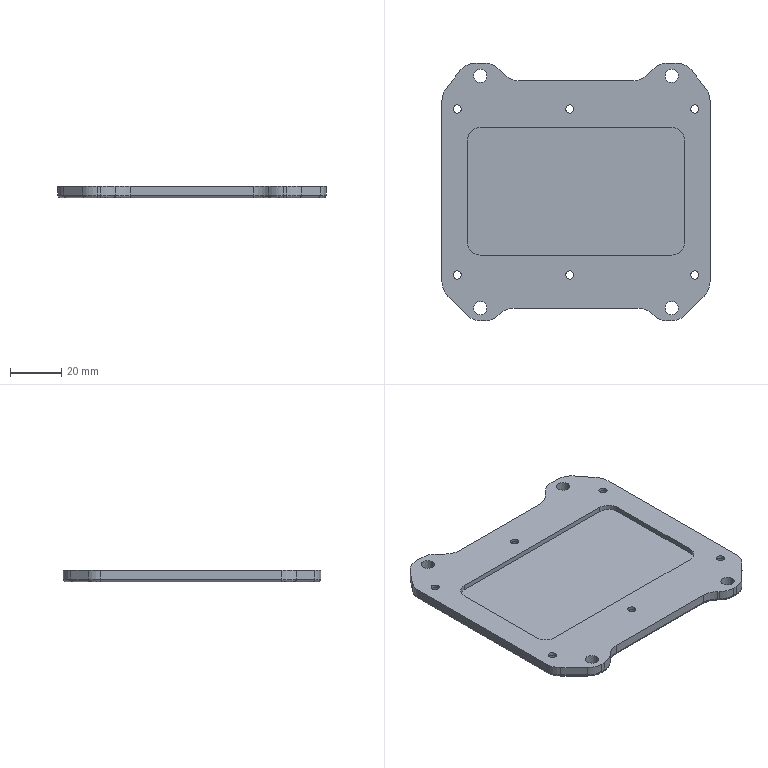NC program | NX | posted with a generic post | part box 105 x 101 x 4.5 mm
Lines 1 to 735 of 30641:
N10 G17 G21 G94 G90
(FLOOR_WALL , TOOL : D80面刀)
N12 T01 M6
N14 G53
N16 G17 G0 G90 X-94.5 Y29.5 S3500 M3
N18 G43 Z20. H1
N20 Z3.
N22 G94 G1 Z0. F800.
N24 X-91.5
N26 X91.5
N28 X94.5
N30 Z3.
N32 G0 Z20.
N34 X-94.5 Y-17.5
N36 Z3.
N38 G1 Z0.
N40 X-91.5
N42 X91.5
N44 X94.5
N46 Z3.
N48 G0 Z20.
N50 M5
(ADAPTIVE_MILLING , TOOL : D8-24-D8-60波刀)
N52 T02 M6
N54 G53
N56 G17 G0 G90 X-71.573 Y-42.037 S5500 M3
N58 G43 Z20. H2
N60 Z-2.5
N62 G94 G1 X-71.424 Y-42.026 Z-3.437 F2500.
N64 X-71.274 Y-42.014 Z-3.808
N66 X-71.125 Y-42.003 Z-4.08
N68 X-70.975 Y-41.991 Z-4.3
N70 X-70.825 Y-41.98 Z-4.484
N72 X-70.676 Y-41.968 Z-4.642
N74 X-70.526 Y-41.957 Z-4.78
N76 X-70.377 Y-41.945 Z-4.9
N78 X-70.227 Y-41.933 Z-5.005
N80 X-70.078 Y-41.922 Z-5.098
N82 X-69.928 Y-41.91 Z-5.179
N84 X-69.779 Y-41.899 Z-5.25
N86 X-69.629 Y-41.887 Z-5.31
N88 X-69.479 Y-41.876 Z-5.362
N90 X-69.33 Y-41.864 Z-5.405
N92 X-69.18 Y-41.853 Z-5.439
N94 X-69.031 Y-41.841 Z-5.466
N96 X-68.881 Y-41.83 Z-5.485
N98 X-68.732 Y-41.818 Z-5.496
N100 X-68.582 Y-41.806 Z-5.5
N102 X-67.206 Y-41.7
N104 G3 X-66.548 Y-41.261 R0.809
N106 X-65.804 Y-38.537 R7.458
N108 X-65.519 Y-31.851 R66.093
N110 G1 X-65.499 Y-23.773
N112 Y60.002
N114 G2 X-64.039 Y62.944 R4.192
N116 X-60.308 Y64.789 R8.351
N118 X-54.802 Y65.406 R27.831
N120 X-42.203 Y65.499 R442.346
N122 G1 X60.002 Y65.498
N124 G2 X62.893 Y64.093 R4.172
N126 X64.754 Y60.451 R8.177
N128 X65.398 Y55.024 R26.448
N130 X65.499 Y42.125 R412.701
N132 G1 X65.498 Y-60.025
N134 G2 X63.974 Y-63.013 R4.208
N136 X60.225 Y-64.813 R8.518
N138 X54.791 Y-65.407 R28.508
N140 X42.267 Y-65.499 R444.885
N142 G1 X-60.075 Y-65.497
N144 G2 X-63.046 Y-63.937 R4.252
N146 X-64.809 Y-60.242 R8.541
N148 X-65.407 Y-54.808 R28.316
N150 X-65.474 Y-43.86 R246.879
N152 X-64.936 Y-39.412 R121.513
N154 G3 X-64.532 Y-31.165 R85.409
N156 G1 X-64.499 Y-21.298
N158 Y57.327
N160 G2 X-62.121 Y61.887 R5.856
N162 X-57.81 Y63.775 R10.676
N164 X-51.701 Y64.405 R34.304
N166 X-39.327 Y64.498 R452.847
N168 G1 X57.451 Y64.495
N170 G2 X61.923 Y62.076 R5.874
N172 X63.803 Y57.684 R10.829
N174 X64.404 Y51.722 R34.892
N176 X64.498 Y38.898 R471.436
N178 G1 X64.495 Y-57.474
N180 G2 X62.056 Y-61.941 R5.867
N182 X57.581 Y-63.824 R10.948
N184 X51.242 Y-64.419 R37.304
N186 X39.242 Y-64.498 R529.27
N188 G1 X-57.474 Y-64.494
N190 G2 X-61.98 Y-62.005 R5.891
N192 X-63.833 Y-57.538 R11.051
N194 X-64.42 Y-51.198 R37.895
N196 X-64.42 Y-44.6 R82.254
N198 X-63.866 Y-38.538 R611.531
N200 G3 X-63.516 Y-28.108 R146.693
N202 G1 X-63.5 Y-19.723
N204 X-63.498 Y55.077
N206 G2 X-60.243 Y61.028 R6.963
N208 X-55.431 Y62.842 R12.911
N210 X-48.863 Y63.417 R42.796
N212 X-36.113 Y63.498 R579.458
N214 G1 X55.037 Y63.497
N216 G2 X60.995 Y60.293 R6.952
N218 X62.834 Y55.476 R12.78
N220 X63.42 Y48.759 R42.92
N222 X63.498 Y36.009 R601.574
N224 G1 X63.496 Y-55.066
N226 G2 X60.318 Y-60.98 R6.936
N228 X55.517 Y-62.825 R12.715
N230 X48.801 Y-63.418 R42.355
N232 X36.051 Y-63.498 R586.161
N234 G1 X-55.024 Y-63.497
N236 G2 X-61.024 Y-60.255 R6.957
N238 X-62.827 Y-55.513 R12.81
N240 X-63.42 Y-48.721 R42.6
N242 X-63.145 Y-41.905 R59.613
N244 G3 X-62.522 Y-27.878 R159.987
N246 G1 X-62.5 Y-19.348
N248 X-62.499 Y52.902
N250 G2 X-61.556 Y57.099 R8.391
N252 X-57.509 Y60.678 R8.645
N254 X-52.23 Y62.055 R17.906
N256 X-44.37 Y62.464 R73.271
N258 G1 X-33.645 Y62.497
N260 X52.876
N262 G2 X56.947 Y61.639 R8.501
N264 X60.602 Y57.673 R8.506
N266 X62.052 Y52.261 R17.664
N268 X62.466 Y44.175 R74.428
N270 G1 X62.497 Y33.45
N272 Y-52.899
N274 G2 X61.594 Y-57.03 R8.453
N276 X57.566 Y-60.652 R8.579
N278 X52.142 Y-62.066 R18.03
N280 X44.056 Y-62.467 R76.552
N282 G1 X34.156 Y-62.497
N284 X-53.049 Y-62.495
N286 G2 X-57.609 Y-61.249 R8.039
N288 X-60.912 Y-56.974 R9.13
N290 X-62.162 Y-51.275 R20.584
N292 X-62.174 Y-42.81 R50.759
N294 G3 X-61.509 Y-24.515 R224.635
N296 G1 X-61.5 Y-17.923
N298 X-61.497 Y51.177
N300 G2 X-60.771 Y55.206 R9.895
N302 X-56.688 Y59.36 R8.698
N304 X-51.166 Y60.972 R17.301
N306 X-43.536 Y61.446 R64.534
N308 X-31.836 Y61.497 R751.309
N310 G1 X51.139 Y61.495
N312 G2 X55.173 Y60.787 R10.005
N314 X59.386 Y56.64 R8.697
N316 X60.968 Y51.19 R17.308
N318 X61.447 Y43.484 R64.617
N320 X61.497 Y31.785 R753.926
N322 G1 X61.496 Y-50.965
N324 G2 X60.883 Y-54.943 R10.636
N326 X56.884 Y-59.256 R8.548
N328 X51.609 Y-60.904 R16.452
N330 X44.358 Y-61.429 R55.962
N332 X31.683 Y-61.497 R748.404
N334 G1 X-51.024 Y-61.496
N336 G2 X-54.927 Y-60.888 R10.484
N338 X-59.27 Y-56.858 R8.529
N340 X-60.937 Y-51.358 R16.573
N342 X-61.165 Y-43.573 R41.521
N344 G3 X-60.609 Y-31.88 R396.831
N346 X-60.501 Y-16.348 R700.345
N348 G1 X-60.499 Y49.302
N350 G2 X-59.991 Y53.227 R12.434
N352 X-55.779 Y58.11 R8.808
N354 X-50.379 Y59.854 R16.601
N356 X-43.056 Y60.418 R54.679
N358 X-29.857 Y60.497 R667.927
N360 G1 X49.051 Y60.496
N362 G2 X52.916 Y60.087 R13.79
N364 X58.015 Y55.95 R8.673
N366 X59.822 Y50.573 R16.141
N368 X60.421 Y42.953 R53.751
N370 X60.497 Y29.454 R720.403
N372 G1 X60.495 Y-49.321
N374 G2 X59.986 Y-53.246 R12.436
N376 X55.796 Y-58.102 R8.781
N378 X50.397 Y-59.85 R16.593
N380 X43. Y-60.419 R54.836
N382 X29.8 Y-60.496 R689.29
N384 G1 X-49.2 Y-60.495
N386 G2 X-53.13 Y-60.023 R12.901
N388 X-58.065 Y-55.863 R8.728
N390 X-59.873 Y-50.02 R16.121
N392 X-60.072 Y-42.681 R43.577
N394 G3 X-59.561 Y-28.982 R418.167
N396 X-59.501 Y-15.523 R806.291
N398 G1 X-59.499 Y47.502
N400 G2 X-59.074 Y51.591 R15.18
N402 X-54.748 Y56.954 R9.023
N404 X-49.153 Y58.816 R16.746
N406 X-41.382 Y59.419 R56.004
N408 X-27.883 Y59.496 R712.08
N410 G1 X47.517 Y59.495
N412 G2 X51.534 Y59.089 R15.327
N414 X56.96 Y54.742 R9.003
N416 X58.818 Y49.142 R16.802
N418 X59.421 Y41.297 R56.559
N420 X59.496 Y27.873 R744.453
N422 G1 X59.495 Y-47.527
N424 G2 X59.086 Y-51.544 R15.168
N426 X54.806 Y-56.92 R8.972
N428 X49.29 Y-58.791 R16.52
N430 X41.822 Y-59.407 R52.883
N432 X27.798 Y-59.496 R628.139
N434 G1 X-47.649 Y-59.494
N436 G2 X-51.661 Y-59.053 R14.513
N438 X-57.004 Y-54.657 R8.998
N440 X-58.782 Y-48.807 R16.044
N442 X-58.98 Y-41.542 R46.704
N444 G3 X-58.502 Y-18.297 R459.973
N446 G1 X-58.501 Y45.327
N448 G2 X-58.246 Y49.513 R22.862
N450 X-53.602 Y55.89 R9.244
N452 X-48.156 Y57.748 R16.848
N454 X-40.691 Y58.395 R51.977
N456 X-26.666 Y58.496 R560.363
N458 G1 X46.051 Y58.494
N460 G2 X50.219 Y58.086 R16.599
N462 X55.907 Y53.575 R9.257
N464 X57.805 Y47.831 R17.256
N466 X58.405 Y40.361 R55.62
N468 X58.496 Y26.337 R626.023
N470 G1 X58.494 Y-46.074
N472 G2 X58.099 Y-50.169 R16.606
N474 X53.618 Y-55.88 R9.235
N476 X48.034 Y-57.769 R16.984
N478 X40.341 Y-58.405 R54.146
N480 X26.317 Y-58.496 R627.916
N482 G1 X-46.008 Y-58.494
N484 G2 X-50.178 Y-58.096 R16.858
N486 X-55.935 Y-53.489 R9.182
N488 X-57.666 Y-47.781 R16.021
N490 X-57.907 Y-40.667 R47.396
N492 G3 X-57.503 Y-16.871 R587.935
N494 G1 X-57.501 Y43.602
N496 G2 X-57.28 Y48.016 R27.888
N498 X-52.454 Y54.846 R9.472
N500 X-46.797 Y56.753 R17.346
N502 X-38.955 Y57.403 R55.282
N504 X-24.631 Y57.495 R635.288
N506 G1 X44.394 Y57.494
N508 G2 X48.647 Y57.154 R19.833
N510 X54.853 Y52.447 R9.46
N512 X56.742 Y46.861 R17.289
N514 X57.403 Y38.87 R54.859
N516 X57.496 Y23.522 R730.661
N518 G1 X57.494 Y-44.374
N520 G2 X57.142 Y-48.7 R19.648
N522 X52.558 Y-54.784 R9.427
N524 X46.837 Y-56.744 R17.19
N526 X39.221 Y-57.394 R53.624
N528 X25.197 Y-57.495 R568.147
N530 G1 X-44.428 Y-57.494
N532 G2 X-48.607 Y-57.162 R19.843
N534 X-54.881 Y-52.308 R9.324
N536 X-56.585 Y-46.511 R16.479
N538 X-56.822 Y-38.946 R52.654
N540 G1 X-56.65 Y-32.25
N542 Y35.735
N544 G3 X-56.515 Y40.291 R49.234
N546 G2 X-56.414 Y45.609 R83.156
N548 X-54.504 Y51.053 R10.169
N550 X-49.5 Y54.678 R11.267
N552 X-43.295 Y56.058 R24.049
N554 X-33.632 Y56.469 R103.808
N556 G1 X-22.907 Y56.495
N558 X43.051 Y56.493
N560 G2 X47.38 Y56.155 R21.05
N562 X53.866 Y51.23 R9.672
N564 X55.758 Y45.48 R17.927
N566 X56.383 Y38.135 R54.805
N568 G1 X56.543 Y37.346
N570 X56.65 Y35.734
N572 Y-35.187
N574 G3 X56.508 Y-40.314 R59.988
N576 G2 X56.395 Y-45.781 R73.953
N578 X54.064 Y-51.595 R9.909
N580 X49. Y-54.863 R11.863
N582 X42.609 Y-56.126 R26.615
N584 X32.568 Y-56.477 R123.888
N586 G1 X23.493 Y-56.495
N588 X-42.907 Y-56.494
N590 G2 X-47.312 Y-56.169 R21.931
N592 X-53.855 Y-51.084 R9.446
N594 X-55.499 Y-45.346 R16.982
N596 X-55.793 Y-39.657 R54.296
N598 G1 X-56.236 Y-38.33
N600 X-56.546 Y-36.771
N602 X-56.65 Y-35.186
N604 Y-32.186
N606 Y-35.186
N608 X-56.546 Y-36.771
N610 X-56.236 Y-38.33
N612 G2 X-55.491 Y-40.714 R19.908
N614 X-54.919 Y-44.963 R132.04
N616 G3 X-53.376 Y-50.273 R17.209
N618 X-46.637 Y-55.369 R9.439
N620 X-41.417 Y-55.847 R28.595
N622 X-31.217 Y-55.895 R689.033
N624 G1 X27.008 Y-55.893
N626 G3 X39.755 Y-55.699 R273.715
N628 X46.81 Y-54.781 R37.053
N630 X52.003 Y-52.351 R13.445
N632 X55.401 Y-46.535 R9.729
N634 X55.857 Y-41.462 R29.876
N636 G2 X55.928 Y-39.239 R28.804
N638 G1 X56.236 Y-38.332
N640 X56.546 Y-36.773
N642 X56.236 Y-38.332
N644 G3 X55.412 Y-40.722 R117.864
N646 X54.741 Y-44.366 R49.802
N648 G2 X53.096 Y-48.929 R12.162
N650 X48.14 Y-52.92 R10.719
N652 X42.038 Y-54.399 R22.462
N654 X32.753 Y-54.855 R91.361
N656 X21.204 Y-54.894 R782.485
N658 G1 X-31.096 Y-54.896
N660 G2 X-41.77 Y-54.804 R328.14
N662 X-46.582 Y-54.113 R18.838
N664 X-52.316 Y-49.083 R9.472
N666 X-53.869 Y-43.999 R19.338
N668 G3 X-54.16 Y-42.572 R13.851
N670 G1 X-55.023 Y-41.26
N672 X-55.725 Y-39.835
N674 X-55.023 Y-41.26
N676 G2 X-53.921 Y-42.957 R19.701
N678 X-52.851 Y-45.957 R30.742
N680 G3 X-50.569 Y-50.321 R13.491
N682 X-45.197 Y-53.554 R9.944
N684 X-40.521 Y-54.177 R25.848
N686 X-38.773 Y-54.546 R22.944
N688 X-33.252 Y-54.449 R26.169
N690 G2 X-25.565 Y-54.296 R124.687
N692 G1 X-22.568 Y-54.295
N694 X24.132 Y-54.293
N696 X32.767 Y-54.255
N698 X34.227 Y-54.546
N700 G3 X38.771 Y-54.546 R23.097
N702 X44.571 Y-53.345 R348.166
N704 X49.655 Y-51.199 R15.013
N706 X53.507 Y-45.86 R10.253
N708 X54.483 Y-42.108 R47.506
N710 G2 X55.022 Y-41.262 R9.389
N712 G1 X55.685 Y-39.917
N714 X55.022 Y-41.262
N716 G3 X52.87 Y-45.061 R19.35
N718 G2 X49.227 Y-49.764 R12.096
N720 X44.819 Y-51.975 R15.096
N722 G1 X43.26 Y-53.023
N724 X41.835 Y-53.725
N726 X40.33 Y-54.236
N728 X41.835 Y-53.725
N730 X43.26 Y-53.023
N732 G3 X45.166 Y-51.663 R16.46
N734 X47.997 Y-49.807 R79.508
N736 X51.931 Y-45.227 R14.088
N738 G1 X52.354 Y-44.515
N740 G3 X54.139 Y-42.584 R23.177
N742 G2 X52.354 Y-44.515 R23.177
N744 G1 X45.777 Y-51.092
N746 X44.582 Y-52.14
N748 X43.26 Y-53.023
N750 X41.835 Y-53.725
N752 X40.33 Y-54.236
N754 X38.771 Y-54.546
N756 G2 X34.227 Y-54.546 R23.097
N758 G1 X32.668 Y-54.236
N760 G3 X29.056 Y-53.492 R11.487
N762 X20.745 Y-53.299 R124.769
N764 G1 X15.8 Y-53.295
N766 X-24.02
N768 G3 X-30.322 Y-53.357 R344.119
N770 X-31.165 Y-53.725 R3.871
N772 G1 X-32.67 Y-54.236
N774 X-34.229 Y-54.546
N776 X-32.67 Y-54.236
N778 X-31.165 Y-53.725
N780 G2 X-28.533 Y-52.928 R6.038
N782 X-22.401 Y-52.705 R65.015
N784 G1 X-17.168 Y-52.695
N786 X17.928 Y-52.696
N788 G2 X27.933 Y-52.849 R191.784
N790 X29.744 Y-53.033 R21.493
N792 G1 X31.163 Y-53.725
N794 X31.66 Y-53.894
N796 X31.163 Y-53.725
N798 G2 X29.3 Y-52.747 R15.885
N800 G3 X26.173 Y-52.005 R9.82
N802 X18.856 Y-51.713 R76.977
N804 G1 X11.525 Y-51.696
N806 X-18.545
N808 G3 X-26.89 Y-51.85 R136.273
N810 X-28.177 Y-52.006 R9.88
N812 G1 X-28.418 Y-52.14
N814 X-29.74 Y-53.023
N816 X-30.345 Y-53.321
N818 X-29.74 Y-53.023
N820 G2 X-28.102 Y-51.918 R81.034
N822 X-25.499 Y-51.333 R8.361
N824 X-18.801 Y-51.107 R75.456
N826 G1 X-11.618 Y-51.096
N828 X14.102 Y-51.098
N830 G2 X24.104 Y-51.269 R187.222
N832 X27.967 Y-51.814 R19.182
N834 X28.417 Y-52.139 R1.667
N836 G1 X29.477 Y-52.847
N838 G2 X27.734 Y-51.558 R11.52
N840 G3 X25.107 Y-50.65 R7.353
N842 X19.028 Y-50.167 R40.671
N844 X6.2 Y-50.096 R733.152
N846 G1 X-15.095 Y-50.099
N848 G3 X-23.901 Y-50.262 R146.918
N850 X-26.735 Y-50.683 R13.581
N852 X-27.223 Y-51.092 R1.744
N854 G1 X-28.351 Y-52.081
N856 X-26.761 Y-50.656
N858 G2 X-24.686 Y-49.948 R5.646
N860 X-21.98 Y-49.65 R27.135
N862 G1 X20.315 Y-49.658
N864 G2 X25.667 Y-50.267 R25.388
N866 X26.742 Y-50.641 R5.005
N868 G1 X27.842 Y-51.635
N870 G3 X26.39 Y-50.352 R43.16
N872 X24.143 Y-49.65 R3.954
N874 G1 X20.018
N876 G3 X19.325 Y-50.051 R0.801
N878 G1 X19.197 Y-50.273
N880 X18.501 Y-51.475 Z-5.411
N882 X18.389 Y-51.61 Z-5.4
N884 G2 X17.84 Y-51.828 R0.805 F15000.
N886 G1 X-19.802
N888 G2 X-20.342 Y-51.619 R0.805
N890 X-20.611 Y-51.225 Z-5.431 R1.54 F2500.
N892 G1 X-21.152 Y-50.284 Z-5.5
N894 X-21.354 Y-49.952
N896 G3 X-21.98 Y-49.65 R0.802
N898 G1 X-24.229 Y-49.654
N900 G3 X-27.016 Y-50.883 R4.063
N902 G2 X-28.418 Y-52.14 R48.219
N904 G1 X-29.74 Y-53.023
N906 X-31.165 Y-53.725
N908 X-32.67 Y-54.236
N910 X-34.229 Y-54.546
N912 G2 X-38.773 Y-54.546 R23.097
N914 X-40.476 Y-54.187 R20.795
N916 X-45.161 Y-52.509 R248.924
N918 X-50.768 Y-47.41 R10.84
N920 X-51.969 Y-44.922 R57.474
N922 G1 X-53.092 Y-43.777
N924 X-54.14 Y-42.582
N926 G3 X-51.714 Y-45.167 R36.342
N928 G2 X-49.982 Y-47.589 R54.24
N930 G3 X-45.186 Y-51.61 R12.743
N932 G1 X-44.583 Y-52.139
N934 X-43.262 Y-53.022
N936 X-41.85 Y-53.718
N938 X-43.262 Y-53.022
N940 X-44.583 Y-52.139
N942 X-45.778 Y-51.091
N944 X-51.824 Y-45.045
N946 G3 X-52.609 Y-44.842 R0.801
N948 G1 X-52.799 Y-44.896
N950 X-54.303 Y-45.326 Z-5.4
N952 G2 X-54.833 Y-45.386 R1.057 F15000.
N954 X-55.344 Y-45.045 R0.804
N956 G1 X-56.159 Y-43.827
N958 X-56.963 Y-42.601
N960 G2 X-58.832 Y-37.018 R13.261
N962 X-58.963 Y-34.683 R21.639
N964 G1 X-59.032 Y34.859
N966 G2 X-58.617 Y35.569 R0.851
N968 G1 X-57.355 Y36.494 Z-5.5 F2500.
N970 X-57.055 Y36.711
N972 X-56.764 Y36.938
N974 G3 X-56.542 Y37.348 R0.813
N976 G2 X-55.993 Y39.748 R25.348
N978 G3 X-55.549 Y43.807 R36.438
N980 G2 X-54.444 Y48.375 R12.828
N982 X-49.521 Y53.147 R10.387
N984 X-43.414 Y54.882 R20.193
N986 X-35.187 Y55.423 R70.107
N988 X-21.162 Y55.495 R792.968
N990 G1 X41.263 Y55.493
N992 G2 X45.823 Y55.218 R26.443
N994 X52.789 Y50.19 R9.829
N996 X54.729 Y44.382 R17.968
N998 X55.113 Y41.635 R158.187
N1000 G1 X55.694 Y40.458
N1002 X56.222 Y38.931
N1004 X56.386 Y38.122
N1006 X56.222 Y38.931
N1008 X55.694 Y40.458
N1010 G2 X54.733 Y42.517 R15.785
N1012 G1 X53.638 Y46.368
N1014 G3 X51.143 Y51.134 R13.622
N1016 X45.289 Y54.411 R9.978
N1018 X40.139 Y54.849 R30.648
N1020 X32.565 Y54.895 R619.068
N1022 G1 X-25.285 Y54.893
N1024 G3 X-38.558 Y54.691 R284.11
N1026 X-45.491 Y53.809 R38.116
N1028 X-50.85 Y51.376 R14.046
N1030 X-54.404 Y45.691 R10.082
N1032 X-55.097 Y41.685 R44.337
N1034 G2 X-55.693 Y40.46 R37.632
N1036 G1 X-56.134 Y39.184
N1038 G2 X-54.766 Y42.219 R12.432
N1040 G3 X-53.67 Y44.967 R24.076
N1042 G2 X-50.421 Y49.869 R11.546
N1044 X-46.678 Y52.072 R13.121
N1046 G1 X-45.193 Y53.062
N1048 G2 X-42.292 Y54.246 R14.216
N1050 G1 X-40.752 Y54.549
N1052 G3 X-43.781 Y53.748 R14.216
N1054 X-46.504 Y52.199 R14.216
N1056 G2 X-48.845 Y50.321 R53.042
N1058 G3 X-52.829 Y45.005 R13.863
N1060 G1 X-53.087 Y44.472
N1062 G3 X-54.859 Y42.062 R24.734
N1064 G2 X-53.087 Y44.472 R24.734
N1066 G1 X-48.741 Y50.005
N1068 G2 X-46.504 Y52.199 R14.219
N1070 X-43.781 Y53.748 R14.216
N1072 X-40.752 Y54.549 R14.216
N1074 G1 X-39.186 Y54.65
N1076 X-35.813
N1078 X-34.227 Y54.546
N1080 G3 X-29.441 Y53.984 R22.659
N1082 X-18.148 Y53.895 R400.93
N1084 G1 X31.527 Y53.894
N1086 X31.749 Y53.924
N1088 X32.67 Y54.236
N1090 X34.229 Y54.546
N1092 X35.814 Y54.65
N1094 X39.187
N1096 G2 X42.294 Y54.246 R14.219
N1098 G3 X44.881 Y53.491 R67.494
N1100 G2 X51.514 Y47.98 R10.799
N1102 X52.897 Y44.732 R26.564
N1104 X54.968 Y41.903 R37.994
N1106 G3 X52.613 Y45.076 R36.865
N1108 G2 X50.908 Y47.804 R104.806
N1110 G3 X47.665 Y51.199 R11.863
N1112 G1 X46.506 Y52.198
N1114 G3 X43.783 Y53.747 R14.216
N1116 G1 X42.858 Y54.057
N1118 X43.783 Y53.747
N1120 G2 X46.506 Y52.198 R14.216
N1122 X48.742 Y50.004 R14.22
N1124 G1 X52.633 Y45.049
N1126 G3 X53.901 Y45.062 R0.8
N1128 X54.041 Y45.743 Z-5.454 R0.841
N1130 G1 X53.911 Y46.58 Z-5.4
N1132 X53.669 Y48.129 F15000.
N1134 X53.623 Y48.296
N1136 X53.544 Y48.45
N1138 X52.778 Y49.582
N1140 G3 X51.74 Y50.739 R8.253
N1142 G1 X50.266 Y52.098
N1144 X48.783 Y53.445
N1146 G3 X46.179 Y55.334 R20.66
N1148 X43.859 Y56.339 R10.212
N1150 X40.993 Y56.912 R17.643
N1152 X39.535 Y56.986 R14.73
N1154 G1 X33.51 Y56.973
N1156 G3 X32.735 Y56.365 R0.8
N1158 G1 X32.708 Y56.258
N1160 X32.331 Y54.74 Z-5.5 F2500.
N1162 X32.283 Y54.55
N1164 X32.226 Y54.362
N1166 G2 X31.749 Y53.924 R0.803
N1168 X28.912 Y53.431 R9.723
N1170 X21.043 Y53.296 R145.933
N1172 G1 X-18.703 Y53.295
N1174 G2 X-29.644 Y53.415 R273.01
N1176 X-30.773 Y53.532 R4.455
N1178 G1 X-31.163 Y53.725
N1180 X-32.668 Y54.236
N1182 X-31.163 Y53.725
N1184 G3 X-29.344 Y52.94 R9.185
N1186 X-25.131 Y52.422 R21.118
N1188 X-15.072 Y52.296 R254.42
N1190 G1 X18.226
N1192 G3 X27.67 Y52.405 R222.151
N1194 X28.984 Y52.542 R6.46
N1196 X29.74 Y53.023 R15.562
N1198 G2 X31.378 Y53.798 R15.642
N1200 G3 X28.914 Y52.475 R11.515
N1202 G2 X26.517 Y51.93 R7.544
N1204 X20.648 Y51.71 R66.929
N1206 G1 X14.07 Y51.696
N1208 X-14.951 Y51.697
N1210 G2 X-25.33 Y51.861 R197.105
N1212 X-28.593 Y52.279 R19.257
N1214 X-29.738 Y53.022 R19.665
N1216 G1 X-30.074 Y53.188
N1218 G2 X-28.708 Y52.333 R9.704
N1220 G3 X-26.177 Y51.286 R5.95
N1222 X-20.755 Y50.784 R33.723
N1224 X-8.698 Y50.696 R472.674
N1226 G1 X15.823 Y50.697
N1228 G3 X24.645 Y50.839 R163.074
N1230 X27.248 Y51.177 R14.762
N1232 G1 X27.445 Y51.286
N1234 G2 X28.979 Y52.515 R9.952
N1236 G3 X27.445 Y51.286 R9.952
N1238 G2 X26.002 Y50.657 R3.386
N1240 X21.522 Y50.181 R23.463
N1242 X12.42 Y50.096 R329.08
N1244 G1 X-11.127 Y50.097
N1246 G2 X-22.114 Y50.265 R215.505
N1248 X-26.598 Y50.892 R21.745
N1250 X-27.307 Y51.166 R2.687
N1252 G1 X-28.417 Y52.139
N1254 G3 X-26.804 Y50.721 R78.533
N1256 X-24.103 Y49.73 R7.54
N1258 X-18.059 Y49.186 R37.896
N1260 X-4.648 Y49.097 R572.443
N1262 G1 X13.796 Y49.099
N1264 G3 X22.595 Y49.28 R138.93
N1266 X25.868 Y49.81 R14.413
N1268 G1 X26.068 Y49.937
N1270 X27.336 Y51.191
N1272 X25.962 Y49.831
N1274 G2 X23.987 Y49.052 R5.073
N1276 X18.915 Y48.575 R30.14
N1278 X8.519 Y48.497 R445.642
N1280 G1 X-5.878
N1282 G2 X-18.931 Y48.636 R347.104
N1284 X-24.426 Y49.29 R28.811
N1286 X-25.937 Y49.821 R6.748
N1288 G1 X-27.061 Y50.93
N1290 X-25.512 Y49.401
N1292 G3 X-22.802 Y48.276 R7.133
N1294 X-17.348 Y47.65 R31.48
N1296 G1 X20.079 Y47.663
N1298 G3 X24.235 Y48.277 R18.769
N1300 X24.939 Y48.808 R2.891
N1302 G1 X26. Y49.869
N1304 G2 X24.252 Y48.26 R13.412
N1306 X22.144 Y47.65 R3.987
N1308 G1 X19.819
N1310 G2 X19.126 Y48.051 R0.801
N1312 G1 X19. Y48.27
N1314 X18.303 Y49.475 Z-5.411
N1316 X18.194 Y49.607 Z-5.4
N1318 G3 X17.641 Y49.828 R0.805 F15000.
N1320 G1 X-15.17
N1322 G3 X-15.707 Y49.621 R0.806
N1324 G1 X-15.837 Y49.468 Z-5.413 F2500.
N1326 X-15.94 Y49.296 Z-5.426
N1328 X-16.523 Y48.291 Z-5.5
N1330 X-16.628 Y48.11
N1332 X-16.743 Y47.936
N1334 G2 X-17.348 Y47.65 R0.803
N1336 X-21.506 Y47.667 R376.199
N1338 X-24.346 Y48.323 R8.989
N1340 X-25.681 Y49.55 R10.157
N1342 G3 X-24.249 Y48.258 R10.381
N1344 X-22.143 Y47.65 R3.988
N1346 G1 X-21.168
N1348 G3 X-20.36 Y48.45 R0.808
N1350 G1 X-20.349 Y49.61
N1352 X-20.348 Y49.76 Z-5.496
N1354 X-20.346 Y49.91 Z-5.485
N1356 X-20.345 Y50.06 Z-5.466
N1358 X-20.344 Y50.21 Z-5.439
N1360 X-20.342 Y50.36 Z-5.405
N1362 X-20.341 Y50.51 Z-5.362
N1364 X-20.339 Y50.66 Z-5.31
N1366 X-20.338 Y50.81 Z-5.25
N1368 X-20.336 Y50.96 Z-5.179
N1370 X-20.335 Y51.11 Z-5.098
N1372 X-20.334 Y51.26 Z-5.005
N1374 X-20.332 Y51.41 Z-4.9
N1376 X-20.331 Y51.56 Z-4.78
N1378 X-20.329 Y51.71 Z-4.642
N1380 X-20.328 Y51.86 Z-4.484
N1382 X-20.327 Y52.01 Z-4.3
N1384 X-20.325 Y52.16 Z-4.08
N1386 X-20.324 Y52.31 Z-3.808
N1388 X-20.322 Y52.46 Z-3.437
N1390 X-20.321 Y52.61 Z-2.5
N1392 G0 Z20.
N1394 M5
(SPOT_DRILLING , TOOL : 倒角D8-90度)
N1396 T05 M6
N1398 G53
N1400 G17 G0 G90 X-46.5 Y32.5 S1600 M3
N1402 G43 Z20. H5
N1404 G94 G81 G98 Z-0.713 F200. R3.
N1406 X-37.5 Y45.5
N1408 X2.5 Y32.5
N1410 X37.5 Y45.5
N1412 X46.5 Y32.5
N1414 Y-32.5
N1416 X37.5 Y-45.5
N1418 X2.5 Y-32.5
N1420 X-37.5 Y-45.5
N1422 X-46.5 Y-32.5
N1424 G80
N1426 M5
(SPOT_DRILLING_1 , TOOL : 钻头D3.3-45-73)
N1428 T07 M6
N1430 G53
N1432 G17 G0 G90 X-46.5 Y32.5 S2500 M3
N1434 G43 Z20. H7
N1436 G94 G81 G98 Z-6. F200. R3.
N1438 X2.5
N1440 X46.5
N1442 Y-32.5
N1444 X2.5
N1446 X-46.5
N1448 G80
N1450 M5